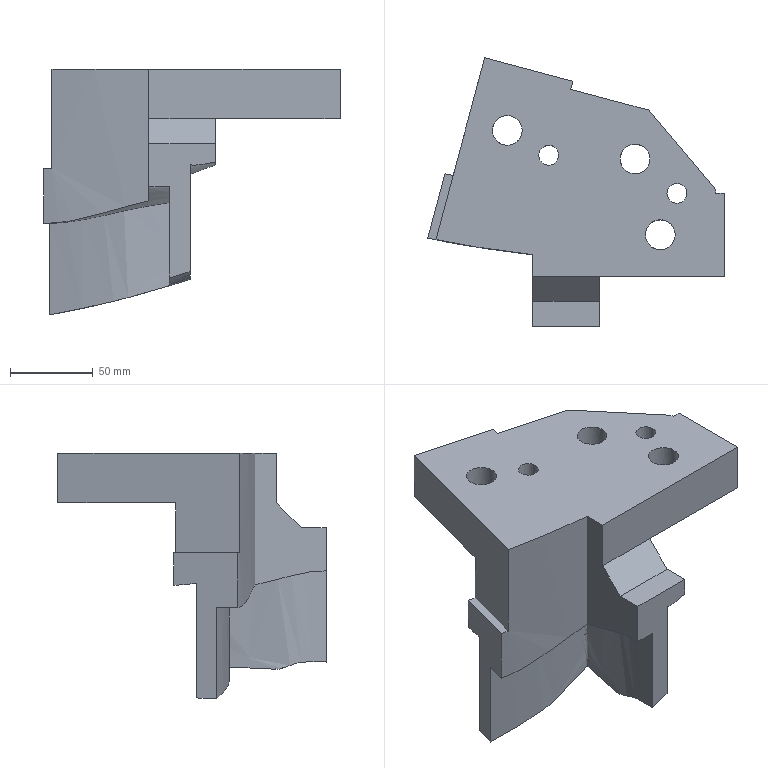Part | NX | features solid 2 | 1 solid | 40 faces | box 178.603 x 161.804 x 148.168 mm | volume 750975 mm3 | plane 21 | spline 11 | cylinder 8 | commonest cylinder face diameters 18 x3 26 x3 12 x2